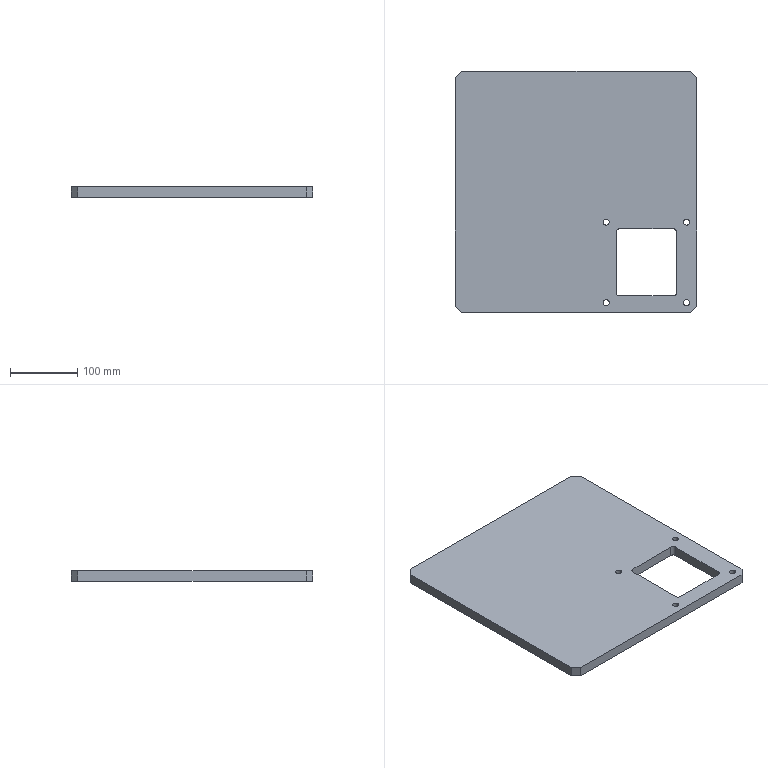Part | SolidWorks | features Chamfer 1, Extrusion 1, Fillet 1, HoleWzd 1, ICE 1 | 1 solid | 26 faces | box 360 x 360 x 15 mm | volume 1802505 mm3 | plane 14 | cylinder 12 | commonest cylinder face diameters 9 x8 10 x4
STEP:
#1=CARTESIAN_POINT('',(160.5,-45.,0.));
#2=VERTEX_POINT('',#1);
#3=CARTESIAN_POINT('',(169.5,-45.,0.));
#4=VERTEX_POINT('',#3);
#5=CARTESIAN_POINT('',(165.,-45.,0.));
#6=DIRECTION('',(0.,0.,1.));
#7=DIRECTION('',(1.,0.,0.));
#8=AXIS2_PLACEMENT_3D('',#5,#6,#7);
#9=CIRCLE('',#8,4.5);
#10=EDGE_CURVE('',#2,#4,#9,.T.);
#11=ORIENTED_EDGE('',*,*,#10,.F.);
#12=CARTESIAN_POINT('',(160.5,-45.,15.));
#13=VERTEX_POINT('',#12);
#14=CARTESIAN_POINT('',(160.5,-45.,15.));
#15=DIRECTION('',(0.,0.,1.));
#16=VECTOR('',#15,1000.);
#17=LINE('',#14,#16);
#18=EDGE_CURVE('',#2,#13,#17,.T.);
#19=ORIENTED_EDGE('',*,*,#18,.T.);
#20=CARTESIAN_POINT('',(169.5,-45.,15.));
#21=VERTEX_POINT('',#20);
#22=CARTESIAN_POINT('',(165.,-45.,15.));
#23=DIRECTION('',(0.,0.,1.));
#24=DIRECTION('',(1.,0.,0.));
#25=AXIS2_PLACEMENT_3D('',#22,#23,#24);
#26=CIRCLE('',#25,4.5);
#27=EDGE_CURVE('',#13,#21,#26,.T.);
#28=ORIENTED_EDGE('',*,*,#27,.T.);
#29=CARTESIAN_POINT('',(169.5,-45.,15.));
#30=DIRECTION('',(0.,0.,1.));
#31=VECTOR('',#30,1000.);
#32=LINE('',#29,#31);
#33=EDGE_CURVE('',#4,#21,#32,.T.);
#34=ORIENTED_EDGE('',*,*,#33,.F.);
#35=EDGE_LOOP('',(#11,#19,#28,#34));
#36=FACE_OUTER_BOUND('',#35,.T.);
#37=CARTESIAN_POINT('',(165.,-45.,15.));
#38=DIRECTION('',(0.,0.,1.));
#39=DIRECTION('',(1.,0.,0.));
#40=AXIS2_PLACEMENT_3D('',#37,#38,#39);
#41=CYLINDRICAL_SURFACE('',#40,4.5);
#42=ADVANCED_FACE('',(#36),#41,.F.);
#43=CARTESIAN_POINT('',(40.5,-45.,0.));
#44=VERTEX_POINT('',#43);
#45=CARTESIAN_POINT('',(49.5,-45.,0.));
#46=VERTEX_POINT('',#45);
#47=CARTESIAN_POINT('',(45.,-45.,0.));
#48=DIRECTION('',(0.,0.,1.));
#49=DIRECTION('',(1.,0.,0.));
#50=AXIS2_PLACEMENT_3D('',#47,#48,#49);
#51=CIRCLE('',#50,4.5);
#52=EDGE_CURVE('',#44,#46,#51,.T.);
#53=ORIENTED_EDGE('',*,*,#52,.F.);
#54=CARTESIAN_POINT('',(40.5,-45.,15.));
#55=VERTEX_POINT('',#54);
#56=CARTESIAN_POINT('',(40.5,-45.,15.));
#57=DIRECTION('',(0.,0.,1.));
#58=VECTOR('',#57,1000.);
#59=LINE('',#56,#58);
#60=EDGE_CURVE('',#44,#55,#59,.T.);
#61=ORIENTED_EDGE('',*,*,#60,.T.);
#62=CARTESIAN_POINT('',(49.5,-45.,15.));
#63=VERTEX_POINT('',#62);
#64=CARTESIAN_POINT('',(45.,-45.,15.));
#65=DIRECTION('',(0.,0.,1.));
#66=DIRECTION('',(1.,0.,0.));
#67=AXIS2_PLACEMENT_3D('',#64,#65,#66);
#68=CIRCLE('',#67,4.5);
#69=EDGE_CURVE('',#55,#63,#68,.T.);
#70=ORIENTED_EDGE('',*,*,#69,.T.);
#71=CARTESIAN_POINT('',(49.5,-45.,15.));
#72=DIRECTION('',(0.,0.,1.));
#73=VECTOR('',#72,1000.);
#74=LINE('',#71,#73);
#75=EDGE_CURVE('',#46,#63,#74,.T.);
#76=ORIENTED_EDGE('',*,*,#75,.F.);
#77=EDGE_LOOP('',(#53,#61,#70,#76));
#78=FACE_OUTER_BOUND('',#77,.T.);
#79=CARTESIAN_POINT('',(45.,-45.,15.));
#80=DIRECTION('',(0.,0.,1.));
#81=DIRECTION('',(1.,0.,0.));
#82=AXIS2_PLACEMENT_3D('',#79,#80,#81);
#83=CYLINDRICAL_SURFACE('',#82,4.5);
#84=ADVANCED_FACE('',(#78),#83,.F.);
#85=CARTESIAN_POINT('',(40.5,-165.,0.));
#86=VERTEX_POINT('',#85);
#87=CARTESIAN_POINT('',(49.5,-165.,0.));
#88=VERTEX_POINT('',#87);
#89=CARTESIAN_POINT('',(45.,-165.,0.));
#90=DIRECTION('',(0.,0.,1.));
#91=DIRECTION('',(1.,0.,0.));
#92=AXIS2_PLACEMENT_3D('',#89,#90,#91);
#93=CIRCLE('',#92,4.5);
#94=EDGE_CURVE('',#86,#88,#93,.T.);
#95=ORIENTED_EDGE('',*,*,#94,.F.);
#96=CARTESIAN_POINT('',(40.5,-165.,15.));
#97=VERTEX_POINT('',#96);
#98=CARTESIAN_POINT('',(40.5,-165.,15.));
#99=DIRECTION('',(0.,0.,1.));
#100=VECTOR('',#99,1000.);
#101=LINE('',#98,#100);
#102=EDGE_CURVE('',#86,#97,#101,.T.);
#103=ORIENTED_EDGE('',*,*,#102,.T.);
#104=CARTESIAN_POINT('',(49.5,-165.,15.));
#105=VERTEX_POINT('',#104);
#106=CARTESIAN_POINT('',(45.,-165.,15.));
#107=DIRECTION('',(0.,0.,1.));
#108=DIRECTION('',(1.,0.,0.));
#109=AXIS2_PLACEMENT_3D('',#106,#107,#108);
#110=CIRCLE('',#109,4.5);
#111=EDGE_CURVE('',#97,#105,#110,.T.);
#112=ORIENTED_EDGE('',*,*,#111,.T.);
#113=CARTESIAN_POINT('',(49.5,-165.,15.));
#114=DIRECTION('',(0.,0.,1.));
#115=VECTOR('',#114,1000.);
#116=LINE('',#113,#115);
#117=EDGE_CURVE('',#88,#105,#116,.T.);
#118=ORIENTED_EDGE('',*,*,#117,.F.);
#119=EDGE_LOOP('',(#95,#103,#112,#118));
#120=FACE_OUTER_BOUND('',#119,.T.);
#121=CARTESIAN_POINT('',(45.,-165.,15.));
#122=DIRECTION('',(0.,0.,1.));
#123=DIRECTION('',(1.,0.,0.));
#124=AXIS2_PLACEMENT_3D('',#121,#122,#123);
#125=CYLINDRICAL_SURFACE('',#124,4.5);
#126=ADVANCED_FACE('',(#120),#125,.F.);
#127=CARTESIAN_POINT('',(160.5,-165.,0.));
#128=VERTEX_POINT('',#127);
#129=CARTESIAN_POINT('',(169.5,-165.,0.));
#130=VERTEX_POINT('',#129);
#131=CARTESIAN_POINT('',(165.,-165.,0.));
#132=DIRECTION('',(0.,0.,1.));
#133=DIRECTION('',(1.,0.,0.));
#134=AXIS2_PLACEMENT_3D('',#131,#132,#133);
#135=CIRCLE('',#134,4.5);
#136=EDGE_CURVE('',#128,#130,#135,.T.);
#137=ORIENTED_EDGE('',*,*,#136,.F.);
#138=CARTESIAN_POINT('',(160.5,-165.,15.));
#139=VERTEX_POINT('',#138);
#140=CARTESIAN_POINT('',(160.5,-165.,15.));
#141=DIRECTION('',(0.,0.,1.));
#142=VECTOR('',#141,1000.);
#143=LINE('',#140,#142);
#144=EDGE_CURVE('',#128,#139,#143,.T.);
#145=ORIENTED_EDGE('',*,*,#144,.T.);
#146=CARTESIAN_POINT('',(169.5,-165.,15.));
#147=VERTEX_POINT('',#146);
#148=CARTESIAN_POINT('',(165.,-165.,15.));
#149=DIRECTION('',(0.,0.,1.));
#150=DIRECTION('',(1.,0.,0.));
#151=AXIS2_PLACEMENT_3D('',#148,#149,#150);
#152=CIRCLE('',#151,4.5);
#153=EDGE_CURVE('',#139,#147,#152,.T.);
#154=ORIENTED_EDGE('',*,*,#153,.T.);
#155=CARTESIAN_POINT('',(169.5,-165.,15.));
#156=DIRECTION('',(0.,0.,1.));
#157=VECTOR('',#156,1000.);
#158=LINE('',#155,#157);
#159=EDGE_CURVE('',#130,#147,#158,.T.);
#160=ORIENTED_EDGE('',*,*,#159,.F.);
#161=EDGE_LOOP('',(#137,#145,#154,#160));
#162=FACE_OUTER_BOUND('',#161,.T.);
#163=CARTESIAN_POINT('',(165.,-165.,15.));
#164=DIRECTION('',(0.,0.,1.));
#165=DIRECTION('',(1.,0.,0.));
#166=AXIS2_PLACEMENT_3D('',#163,#164,#165);
#167=CYLINDRICAL_SURFACE('',#166,4.5);
#168=ADVANCED_FACE('',(#162),#167,.F.);
#169=CARTESIAN_POINT('',(-180.,170.,0.));
#170=VERTEX_POINT('',#169);
#171=CARTESIAN_POINT('',(-180.,-170.,0.));
#172=VERTEX_POINT('',#171);
#173=CARTESIAN_POINT('',(-180.,180.,0.));
#174=DIRECTION('',(0.,-1.,0.));
#175=VECTOR('',#174,1000.);
#176=LINE('',#173,#175);
#177=EDGE_CURVE('',#170,#172,#176,.T.);
#178=ORIENTED_EDGE('',*,*,#177,.T.);
#179=CARTESIAN_POINT('',(-180.,-170.,15.));
#180=VERTEX_POINT('',#179);
#181=CARTESIAN_POINT('',(-180.,-170.,15.));
#182=DIRECTION('',(0.,0.,1.));
#183=VECTOR('',#182,1000.);
#184=LINE('',#181,#183);
#185=EDGE_CURVE('',#172,#180,#184,.T.);
#186=ORIENTED_EDGE('',*,*,#185,.T.);
#187=CARTESIAN_POINT('',(-180.,170.,15.));
#188=VERTEX_POINT('',#187);
#189=CARTESIAN_POINT('',(-180.,180.,15.));
#190=DIRECTION('',(0.,-1.,0.));
#191=VECTOR('',#190,1000.);
#192=LINE('',#189,#191);
#193=EDGE_CURVE('',#188,#180,#192,.T.);
#194=ORIENTED_EDGE('',*,*,#193,.F.);
#195=CARTESIAN_POINT('',(-180.,170.,0.));
#196=DIRECTION('',(0.,0.,-1.));
#197=VECTOR('',#196,1000.);
#198=LINE('',#195,#197);
#199=EDGE_CURVE('',#188,#170,#198,.T.);
#200=ORIENTED_EDGE('',*,*,#199,.T.);
#201=EDGE_LOOP('',(#178,#186,#194,#200));
#202=FACE_OUTER_BOUND('',#201,.T.);
#203=CARTESIAN_POINT('',(-180.,180.,15.));
#204=DIRECTION('',(1.,0.,0.));
#205=DIRECTION('',(0.,1.,0.));
#206=AXIS2_PLACEMENT_3D('',#203,#204,#205);
#207=PLANE('',#206);
#208=ADVANCED_FACE('',(#202),#207,.F.);
#209=CARTESIAN_POINT('',(-170.,-180.,15.));
#210=VERTEX_POINT('',#209);
#211=CARTESIAN_POINT('',(170.,-180.,15.));
#212=VERTEX_POINT('',#211);
#213=CARTESIAN_POINT('',(-180.,-180.,15.));
#214=DIRECTION('',(1.,0.,0.));
#215=VECTOR('',#214,1000.);
#216=LINE('',#213,#215);
#217=EDGE_CURVE('',#210,#212,#216,.T.);
#218=ORIENTED_EDGE('',*,*,#217,.F.);
#219=CARTESIAN_POINT('',(-170.,-180.,0.));
#220=VERTEX_POINT('',#219);
#221=CARTESIAN_POINT('',(-170.,-180.,15.));
#222=DIRECTION('',(0.,0.,-1.));
#223=VECTOR('',#222,1000.);
#224=LINE('',#221,#223);
#225=EDGE_CURVE('',#210,#220,#224,.T.);
#226=ORIENTED_EDGE('',*,*,#225,.T.);
#227=CARTESIAN_POINT('',(170.,-180.,0.));
#228=VERTEX_POINT('',#227);
#229=CARTESIAN_POINT('',(-180.,-180.,0.));
#230=DIRECTION('',(1.,0.,0.));
#231=VECTOR('',#230,1000.);
#232=LINE('',#229,#231);
#233=EDGE_CURVE('',#220,#228,#232,.T.);
#234=ORIENTED_EDGE('',*,*,#233,.T.);
#235=CARTESIAN_POINT('',(170.,-180.,15.));
#236=DIRECTION('',(0.,0.,1.));
#237=VECTOR('',#236,1000.);
#238=LINE('',#235,#237);
#239=EDGE_CURVE('',#228,#212,#238,.T.);
#240=ORIENTED_EDGE('',*,*,#239,.T.);
#241=EDGE_LOOP('',(#218,#226,#234,#240));
#242=FACE_OUTER_BOUND('',#241,.T.);
#243=CARTESIAN_POINT('',(-180.,-180.,15.));
#244=DIRECTION('',(0.,1.,0.));
#245=DIRECTION('',(0.,0.,1.));
#246=AXIS2_PLACEMENT_3D('',#243,#244,#245);
#247=PLANE('',#246);
#248=ADVANCED_FACE('',(#242),#247,.F.);
#249=CARTESIAN_POINT('',(180.,170.,15.));
#250=VERTEX_POINT('',#249);
#251=CARTESIAN_POINT('',(180.,-170.,15.));
#252=VERTEX_POINT('',#251);
#253=CARTESIAN_POINT('',(180.,180.,15.));
#254=DIRECTION('',(0.,-1.,0.));
#255=VECTOR('',#254,1000.);
#256=LINE('',#253,#255);
#257=EDGE_CURVE('',#250,#252,#256,.T.);
#258=ORIENTED_EDGE('',*,*,#257,.T.);
#259=CARTESIAN_POINT('',(180.,-170.,0.));
#260=VERTEX_POINT('',#259);
#261=CARTESIAN_POINT('',(180.,-170.,0.));
#262=DIRECTION('',(0.,0.,-1.));
#263=VECTOR('',#262,1000.);
#264=LINE('',#261,#263);
#265=EDGE_CURVE('',#252,#260,#264,.T.);
#266=ORIENTED_EDGE('',*,*,#265,.T.);
#267=CARTESIAN_POINT('',(180.,170.,0.));
#268=VERTEX_POINT('',#267);
#269=CARTESIAN_POINT('',(180.,180.,0.));
#270=DIRECTION('',(0.,-1.,0.));
#271=VECTOR('',#270,1000.);
#272=LINE('',#269,#271);
#273=EDGE_CURVE('',#268,#260,#272,.T.);
#274=ORIENTED_EDGE('',*,*,#273,.F.);
#275=CARTESIAN_POINT('',(180.,170.,15.));
#276=DIRECTION('',(0.,0.,1.));
#277=VECTOR('',#276,1000.);
#278=LINE('',#275,#277);
#279=EDGE_CURVE('',#268,#250,#278,.T.);
#280=ORIENTED_EDGE('',*,*,#279,.T.);
#281=EDGE_LOOP('',(#258,#266,#274,#280));
#282=FACE_OUTER_BOUND('',#281,.T.);
#283=CARTESIAN_POINT('',(180.,180.,15.));
#284=DIRECTION('',(1.,0.,0.));
#285=DIRECTION('',(0.,1.,0.));
#286=AXIS2_PLACEMENT_3D('',#283,#284,#285);
#287=PLANE('',#286);
#288=ADVANCED_FACE('',(#282),#287,.T.);
#289=CARTESIAN_POINT('',(-170.,180.,15.));
#290=VERTEX_POINT('',#289);
#291=CARTESIAN_POINT('',(170.,180.,15.));
#292=VERTEX_POINT('',#291);
#293=CARTESIAN_POINT('',(-180.,180.,15.));
#294=DIRECTION('',(1.,0.,0.));
#295=VECTOR('',#294,1000.);
#296=LINE('',#293,#295);
#297=EDGE_CURVE('',#290,#292,#296,.T.);
#298=ORIENTED_EDGE('',*,*,#297,.T.);
#299=CARTESIAN_POINT('',(170.,180.,0.));
#300=VERTEX_POINT('',#299);
#301=CARTESIAN_POINT('',(170.,180.,15.));
#302=DIRECTION('',(0.,0.,-1.));
#303=VECTOR('',#302,1000.);
#304=LINE('',#301,#303);
#305=EDGE_CURVE('',#292,#300,#304,.T.);
#306=ORIENTED_EDGE('',*,*,#305,.T.);
#307=CARTESIAN_POINT('',(-170.,180.,0.));
#308=VERTEX_POINT('',#307);
#309=CARTESIAN_POINT('',(-180.,180.,0.));
#310=DIRECTION('',(1.,0.,0.));
#311=VECTOR('',#310,1000.);
#312=LINE('',#309,#311);
#313=EDGE_CURVE('',#308,#300,#312,.T.);
#314=ORIENTED_EDGE('',*,*,#313,.F.);
#315=CARTESIAN_POINT('',(-170.,180.,15.));
#316=DIRECTION('',(0.,0.,1.));
#317=VECTOR('',#316,1000.);
#318=LINE('',#315,#317);
#319=EDGE_CURVE('',#308,#290,#318,.T.);
#320=ORIENTED_EDGE('',*,*,#319,.T.);
#321=EDGE_LOOP('',(#298,#306,#314,#320));
#322=FACE_OUTER_BOUND('',#321,.T.);
#323=CARTESIAN_POINT('',(-180.,180.,15.));
#324=DIRECTION('',(0.,1.,0.));
#325=DIRECTION('',(0.,0.,1.));
#326=AXIS2_PLACEMENT_3D('',#323,#324,#325);
#327=PLANE('',#326);
#328=ADVANCED_FACE('',(#322),#327,.T.);
#329=CARTESIAN_POINT('',(150.,-150.,15.));
#330=VERTEX_POINT('',#329);
#331=CARTESIAN_POINT('',(150.,-60.,15.));
#332=VERTEX_POINT('',#331);
#333=CARTESIAN_POINT('',(150.,-55.,15.));
#334=DIRECTION('',(0.,1.,0.));
#335=VECTOR('',#334,1000.);
#336=LINE('',#333,#335);
#337=EDGE_CURVE('',#330,#332,#336,.T.);
#338=ORIENTED_EDGE('',*,*,#337,.F.);
#339=CARTESIAN_POINT('',(145.,-155.,15.));
#340=VERTEX_POINT('',#339);
#341=CARTESIAN_POINT('',(145.,-150.,15.));
#342=DIRECTION('',(0.,0.,-1.));
#343=DIRECTION('',(1.,0.,0.));
#344=AXIS2_PLACEMENT_3D('',#341,#342,#343);
#345=CIRCLE('',#344,5.);
#346=EDGE_CURVE('',#330,#340,#345,.T.);
#347=ORIENTED_EDGE('',*,*,#346,.T.);
#348=CARTESIAN_POINT('',(65.,-155.,15.));
#349=VERTEX_POINT('',#348);
#350=CARTESIAN_POINT('',(60.,-155.,15.));
#351=DIRECTION('',(1.,0.,0.));
#352=VECTOR('',#351,1000.);
#353=LINE('',#350,#352);
#354=EDGE_CURVE('',#349,#340,#353,.T.);
#355=ORIENTED_EDGE('',*,*,#354,.F.);
#356=CARTESIAN_POINT('',(60.,-150.,15.));
#357=VERTEX_POINT('',#356);
#358=CARTESIAN_POINT('',(65.,-150.,15.));
#359=DIRECTION('',(0.,0.,-1.));
#360=DIRECTION('',(1.,0.,0.));
#361=AXIS2_PLACEMENT_3D('',#358,#359,#360);
#362=CIRCLE('',#361,5.);
#363=EDGE_CURVE('',#349,#357,#362,.T.);
#364=ORIENTED_EDGE('',*,*,#363,.T.);
#365=CARTESIAN_POINT('',(60.,-60.,15.));
#366=VERTEX_POINT('',#365);
#367=CARTESIAN_POINT('',(60.,-55.,15.));
#368=DIRECTION('',(0.,-1.,0.));
#369=VECTOR('',#368,1000.);
#370=LINE('',#367,#369);
#371=EDGE_CURVE('',#366,#357,#370,.T.);
#372=ORIENTED_EDGE('',*,*,#371,.F.);
#373=CARTESIAN_POINT('',(65.,-55.,15.));
#374=VERTEX_POINT('',#373);
#375=CARTESIAN_POINT('',(65.,-60.,15.));
#376=DIRECTION('',(0.,0.,-1.));
#377=DIRECTION('',(1.,0.,0.));
#378=AXIS2_PLACEMENT_3D('',#375,#376,#377);
#379=CIRCLE('',#378,5.);
#380=EDGE_CURVE('',#366,#374,#379,.T.);
#381=ORIENTED_EDGE('',*,*,#380,.T.);
#382=CARTESIAN_POINT('',(145.,-55.,15.));
#383=VERTEX_POINT('',#382);
#384=CARTESIAN_POINT('',(60.,-55.,15.));
#385=DIRECTION('',(-1.,0.,0.));
#386=VECTOR('',#385,1000.);
#387=LINE('',#384,#386);
#388=EDGE_CURVE('',#383,#374,#387,.T.);
#389=ORIENTED_EDGE('',*,*,#388,.F.);
#390=CARTESIAN_POINT('',(145.,-60.,15.));
#391=DIRECTION('',(0.,0.,-1.));
#392=DIRECTION('',(1.,0.,0.));
#393=AXIS2_PLACEMENT_3D('',#390,#391,#392);
#394=CIRCLE('',#393,5.);
#395=EDGE_CURVE('',#383,#332,#394,.T.);
#396=ORIENTED_EDGE('',*,*,#395,.T.);
#397=EDGE_LOOP('',(#338,#347,#355,#364,#372,#381,#389,#396));
#398=FACE_BOUND('',#397,.T.);
#399=CARTESIAN_POINT('',(165.,-45.,15.));
#400=DIRECTION('',(0.,0.,1.));
#401=DIRECTION('',(1.,0.,0.));
#402=AXIS2_PLACEMENT_3D('',#399,#400,#401);
#403=CIRCLE('',#402,4.5);
#404=EDGE_CURVE('',#21,#13,#403,.T.);
#405=ORIENTED_EDGE('',*,*,#404,.F.);
#406=ORIENTED_EDGE('',*,*,#27,.F.);
#407=EDGE_LOOP('',(#405,#406));
#408=FACE_BOUND('',#407,.T.);
#409=CARTESIAN_POINT('',(45.,-45.,15.));
#410=DIRECTION('',(0.,0.,1.));
#411=DIRECTION('',(1.,0.,0.));
#412=AXIS2_PLACEMENT_3D('',#409,#410,#411);
#413=CIRCLE('',#412,4.5);
#414=EDGE_CURVE('',#63,#55,#413,.T.);
#415=ORIENTED_EDGE('',*,*,#414,.F.);
#416=ORIENTED_EDGE('',*,*,#69,.F.);
#417=EDGE_LOOP('',(#415,#416));
#418=FACE_BOUND('',#417,.T.);
#419=CARTESIAN_POINT('',(45.,-165.,15.));
#420=DIRECTION('',(0.,0.,1.));
#421=DIRECTION('',(1.,0.,0.));
#422=AXIS2_PLACEMENT_3D('',#419,#420,#421);
#423=CIRCLE('',#422,4.5);
#424=EDGE_CURVE('',#105,#97,#423,.T.);
#425=ORIENTED_EDGE('',*,*,#424,.F.);
#426=ORIENTED_EDGE('',*,*,#111,.F.);
#427=EDGE_LOOP('',(#425,#426));
#428=FACE_BOUND('',#427,.T.);
#429=CARTESIAN_POINT('',(165.,-165.,15.));
#430=DIRECTION('',(0.,0.,1.));
#431=DIRECTION('',(1.,0.,0.));
#432=AXIS2_PLACEMENT_3D('',#429,#430,#431);
#433=CIRCLE('',#432,4.5);
#434=EDGE_CURVE('',#147,#139,#433,.T.);
#435=ORIENTED_EDGE('',*,*,#434,.F.);
#436=ORIENTED_EDGE('',*,*,#153,.F.);
#437=EDGE_LOOP('',(#435,#436));
#438=FACE_BOUND('',#437,.T.);
#439=ORIENTED_EDGE('',*,*,#193,.T.);
#440=CARTESIAN_POINT('',(-175.,-175.,15.));
#441=DIRECTION('',(0.7071,-0.7071,0.));
#442=VECTOR('',#441,1000.);
#443=LINE('',#440,#442);
#444=EDGE_CURVE('',#180,#210,#443,.T.);
#445=ORIENTED_EDGE('',*,*,#444,.T.);
#446=ORIENTED_EDGE('',*,*,#217,.T.);
#447=CARTESIAN_POINT('',(175.,-175.,15.));
#448=DIRECTION('',(0.7071,0.7071,0.));
#449=VECTOR('',#448,1000.);
#450=LINE('',#447,#449);
#451=EDGE_CURVE('',#212,#252,#450,.T.);
#452=ORIENTED_EDGE('',*,*,#451,.T.);
#453=ORIENTED_EDGE('',*,*,#257,.F.);
#454=CARTESIAN_POINT('',(175.,175.,15.));
#455=DIRECTION('',(-0.7071,0.7071,0.));
#456=VECTOR('',#455,1000.);
#457=LINE('',#454,#456);
#458=EDGE_CURVE('',#250,#292,#457,.T.);
#459=ORIENTED_EDGE('',*,*,#458,.T.);
#460=ORIENTED_EDGE('',*,*,#297,.F.);
#461=CARTESIAN_POINT('',(-175.,175.,15.));
#462=DIRECTION('',(-0.7071,-0.7071,0.));
#463=VECTOR('',#462,1000.);
#464=LINE('',#461,#463);
#465=EDGE_CURVE('',#290,#188,#464,.T.);
#466=ORIENTED_EDGE('',*,*,#465,.T.);
#467=EDGE_LOOP('',(#439,#445,#446,#452,#453,#459,#460,#466));
#468=FACE_OUTER_BOUND('',#467,.T.);
#469=CARTESIAN_POINT('',(0.,0.,15.));
#470=DIRECTION('',(0.,0.,1.));
#471=DIRECTION('',(1.,0.,0.));
#472=AXIS2_PLACEMENT_3D('',#469,#470,#471);
#473=PLANE('',#472);
#474=ADVANCED_FACE('',(#398,#408,#418,#428,#438,#468),#473,.T.);
#475=CARTESIAN_POINT('',(60.,-60.,0.));
#476=VERTEX_POINT('',#475);
#477=CARTESIAN_POINT('',(60.,-150.,0.));
#478=VERTEX_POINT('',#477);
#479=CARTESIAN_POINT('',(60.,-55.,0.));
#480=DIRECTION('',(0.,-1.,0.));
#481=VECTOR('',#480,1000.);
#482=LINE('',#479,#481);
#483=EDGE_CURVE('',#476,#478,#482,.T.);
#484=ORIENTED_EDGE('',*,*,#483,.T.);
#485=CARTESIAN_POINT('',(65.,-155.,0.));
#486=VERTEX_POINT('',#485);
#487=CARTESIAN_POINT('',(65.,-150.,0.));
#488=DIRECTION('',(0.,0.,1.));
#489=DIRECTION('',(1.,0.,0.));
#490=AXIS2_PLACEMENT_3D('',#487,#488,#489);
#491=CIRCLE('',#490,5.);
#492=EDGE_CURVE('',#478,#486,#491,.T.);
#493=ORIENTED_EDGE('',*,*,#492,.T.);
#494=CARTESIAN_POINT('',(145.,-155.,0.));
#495=VERTEX_POINT('',#494);
#496=CARTESIAN_POINT('',(60.,-155.,0.));
#497=DIRECTION('',(1.,0.,0.));
#498=VECTOR('',#497,1000.);
#499=LINE('',#496,#498);
#500=EDGE_CURVE('',#486,#495,#499,.T.);
#501=ORIENTED_EDGE('',*,*,#500,.T.);
#502=CARTESIAN_POINT('',(150.,-150.,0.));
#503=VERTEX_POINT('',#502);
#504=CARTESIAN_POINT('',(145.,-150.,0.));
#505=DIRECTION('',(0.,0.,1.));
#506=DIRECTION('',(1.,0.,0.));
#507=AXIS2_PLACEMENT_3D('',#504,#505,#506);
#508=CIRCLE('',#507,5.);
#509=EDGE_CURVE('',#495,#503,#508,.T.);
#510=ORIENTED_EDGE('',*,*,#509,.T.);
#511=CARTESIAN_POINT('',(150.,-60.,0.));
#512=VERTEX_POINT('',#511);
#513=CARTESIAN_POINT('',(150.,-55.,0.));
#514=DIRECTION('',(0.,1.,0.));
#515=VECTOR('',#514,1000.);
#516=LINE('',#513,#515);
#517=EDGE_CURVE('',#503,#512,#516,.T.);
#518=ORIENTED_EDGE('',*,*,#517,.T.);
#519=CARTESIAN_POINT('',(145.,-55.,0.));
#520=VERTEX_POINT('',#519);
#521=CARTESIAN_POINT('',(145.,-60.,0.));
#522=DIRECTION('',(0.,0.,1.));
#523=DIRECTION('',(1.,0.,0.));
#524=AXIS2_PLACEMENT_3D('',#521,#522,#523);
#525=CIRCLE('',#524,5.);
#526=EDGE_CURVE('',#512,#520,#525,.T.);
#527=ORIENTED_EDGE('',*,*,#526,.T.);
#528=CARTESIAN_POINT('',(65.,-55.,0.));
#529=VERTEX_POINT('',#528);
#530=CARTESIAN_POINT('',(60.,-55.,0.));
#531=DIRECTION('',(-1.,0.,0.));
#532=VECTOR('',#531,1000.);
#533=LINE('',#530,#532);
#534=EDGE_CURVE('',#520,#529,#533,.T.);
#535=ORIENTED_EDGE('',*,*,#534,.T.);
#536=CARTESIAN_POINT('',(65.,-60.,0.));
#537=DIRECTION('',(0.,0.,1.));
#538=DIRECTION('',(1.,0.,0.));
#539=AXIS2_PLACEMENT_3D('',#536,#537,#538);
#540=CIRCLE('',#539,5.);
#541=EDGE_CURVE('',#529,#476,#540,.T.);
#542=ORIENTED_EDGE('',*,*,#541,.T.);
#543=EDGE_LOOP('',(#484,#493,#501,#510,#518,#527,#535,#542));
#544=FACE_BOUND('',#543,.T.);
#545=CARTESIAN_POINT('',(165.,-45.,0.));
#546=DIRECTION('',(0.,0.,1.));
#547=DIRECTION('',(1.,0.,0.));
#548=AXIS2_PLACEMENT_3D('',#545,#546,#547);
#549=CIRCLE('',#548,4.5);
#550=EDGE_CURVE('',#4,#2,#549,.T.);
#551=ORIENTED_EDGE('',*,*,#550,.T.);
#552=ORIENTED_EDGE('',*,*,#10,.T.);
#553=EDGE_LOOP('',(#551,#552));
#554=FACE_BOUND('',#553,.T.);
#555=CARTESIAN_POINT('',(45.,-45.,0.));
#556=DIRECTION('',(0.,0.,1.));
#557=DIRECTION('',(1.,0.,0.));
#558=AXIS2_PLACEMENT_3D('',#555,#556,#557);
#559=CIRCLE('',#558,4.5);
#560=EDGE_CURVE('',#46,#44,#559,.T.);
#561=ORIENTED_EDGE('',*,*,#560,.T.);
#562=ORIENTED_EDGE('',*,*,#52,.T.);
#563=EDGE_LOOP('',(#561,#562));
#564=FACE_BOUND('',#563,.T.);
#565=CARTESIAN_POINT('',(45.,-165.,0.));
#566=DIRECTION('',(0.,0.,1.));
#567=DIRECTION('',(1.,0.,0.));
#568=AXIS2_PLACEMENT_3D('',#565,#566,#567);
#569=CIRCLE('',#568,4.5);
#570=EDGE_CURVE('',#88,#86,#569,.T.);
#571=ORIENTED_EDGE('',*,*,#570,.T.);
#572=ORIENTED_EDGE('',*,*,#94,.T.);
#573=EDGE_LOOP('',(#571,#572));
#574=FACE_BOUND('',#573,.T.);
#575=CARTESIAN_POINT('',(165.,-165.,0.));
#576=DIRECTION('',(0.,0.,1.));
#577=DIRECTION('',(1.,0.,0.));
#578=AXIS2_PLACEMENT_3D('',#575,#576,#577);
#579=CIRCLE('',#578,4.5);
#580=EDGE_CURVE('',#130,#128,#579,.T.);
#581=ORIENTED_EDGE('',*,*,#580,.T.);
#582=ORIENTED_EDGE('',*,*,#136,.T.);
#583=EDGE_LOOP('',(#581,#582));
#584=FACE_BOUND('',#583,.T.);
#585=ORIENTED_EDGE('',*,*,#233,.F.);
#586=CARTESIAN_POINT('',(-170.,-180.,0.));
#587=DIRECTION('',(-0.7071,0.7071,0.));
#588=VECTOR('',#587,1000.);
#589=LINE('',#586,#588);
#590=EDGE_CURVE('',#220,#172,#589,.T.);
#591=ORIENTED_EDGE('',*,*,#590,.T.);
#592=ORIENTED_EDGE('',*,*,#177,.F.);
#593=CARTESIAN_POINT('',(-180.,170.,0.));
#594=DIRECTION('',(0.7071,0.7071,0.));
#595=VECTOR('',#594,1000.);
#596=LINE('',#593,#595);
#597=EDGE_CURVE('',#170,#308,#596,.T.);
#598=ORIENTED_EDGE('',*,*,#597,.T.);
#599=ORIENTED_EDGE('',*,*,#313,.T.);
#600=CARTESIAN_POINT('',(170.,180.,0.));
#601=DIRECTION('',(0.7071,-0.7071,0.));
#602=VECTOR('',#601,1000.);
#603=LINE('',#600,#602);
#604=EDGE_CURVE('',#300,#268,#603,.T.);
#605=ORIENTED_EDGE('',*,*,#604,.T.);
#606=ORIENTED_EDGE('',*,*,#273,.T.);
#607=CARTESIAN_POINT('',(180.,-170.,0.));
#608=DIRECTION('',(-0.7071,-0.7071,0.));
#609=VECTOR('',#608,1000.);
#610=LINE('',#607,#609);
#611=EDGE_CURVE('',#260,#228,#610,.T.);
#612=ORIENTED_EDGE('',*,*,#611,.T.);
#613=EDGE_LOOP('',(#585,#591,#592,#598,#599,#605,#606,#612));
#614=FACE_OUTER_BOUND('',#613,.T.);
#615=CARTESIAN_POINT('',(0.,0.,0.));
#616=DIRECTION('',(0.,0.,1.));
#617=DIRECTION('',(1.,0.,0.));
#618=AXIS2_PLACEMENT_3D('',#615,#616,#617);
#619=PLANE('',#618);
#620=ADVANCED_FACE('',(#544,#554,#564,#574,#584,#614),#619,.F.);
#621=ORIENTED_EDGE('',*,*,#444,.F.);
#622=ORIENTED_EDGE('',*,*,#185,.F.);
#623=ORIENTED_EDGE('',*,*,#590,.F.);
#624=ORIENTED_EDGE('',*,*,#225,.F.);
#625=EDGE_LOOP('',(#621,#622,#623,#624));
#626=FACE_OUTER_BOUND('',#625,.T.);
#627=CARTESIAN_POINT('',(-170.,-180.,15.));
#628=DIRECTION('',(0.7071,0.7071,0.));
#629=DIRECTION('',(0.,0.,-1.));
#630=AXIS2_PLACEMENT_3D('',#627,#628,#629);
#631=PLANE('',#630);
#632=ADVANCED_FACE('',(#626),#631,.F.);
#633=ORIENTED_EDGE('',*,*,#451,.F.);
#634=ORIENTED_EDGE('',*,*,#239,.F.);
#635=ORIENTED_EDGE('',*,*,#611,.F.);
#636=ORIENTED_EDGE('',*,*,#265,.F.);
#637=EDGE_LOOP('',(#633,#634,#635,#636));
#638=FACE_OUTER_BOUND('',#637,.T.);
#639=CARTESIAN_POINT('',(180.,-170.,15.));
#640=DIRECTION('',(0.7071,-0.7071,0.));
#641=DIRECTION('',(0.,0.,1.));
#642=AXIS2_PLACEMENT_3D('',#639,#640,#641);
#643=PLANE('',#642);
#644=ADVANCED_FACE('',(#638),#643,.T.);
#645=ORIENTED_EDGE('',*,*,#458,.F.);
#646=ORIENTED_EDGE('',*,*,#279,.F.);
#647=ORIENTED_EDGE('',*,*,#604,.F.);
#648=ORIENTED_EDGE('',*,*,#305,.F.);
#649=EDGE_LOOP('',(#645,#646,#647,#648));
#650=FACE_OUTER_BOUND('',#649,.T.);
#651=CARTESIAN_POINT('',(170.,180.,15.));
#652=DIRECTION('',(-0.7071,-0.7071,0.));
#653=DIRECTION('',(0.,0.,-1.));
#654=AXIS2_PLACEMENT_3D('',#651,#652,#653);
#655=PLANE('',#654);
#656=ADVANCED_FACE('',(#650),#655,.F.);
#657=ORIENTED_EDGE('',*,*,#465,.F.);
#658=ORIENTED_EDGE('',*,*,#319,.F.);
#659=ORIENTED_EDGE('',*,*,#597,.F.);
#660=ORIENTED_EDGE('',*,*,#199,.F.);
#661=EDGE_LOOP('',(#657,#658,#659,#660));
#662=FACE_OUTER_BOUND('',#661,.T.);
#663=CARTESIAN_POINT('',(-180.,170.,15.));
#664=DIRECTION('',(-0.7071,0.7071,0.));
#665=DIRECTION('',(0.,0.,1.));
#666=AXIS2_PLACEMENT_3D('',#663,#664,#665);
#667=PLANE('',#666);
#668=ADVANCED_FACE('',(#662),#667,.T.);
#669=ORIENTED_EDGE('',*,*,#144,.F.);
#670=ORIENTED_EDGE('',*,*,#580,.F.);
#671=ORIENTED_EDGE('',*,*,#159,.T.);
#672=ORIENTED_EDGE('',*,*,#434,.T.);
#673=EDGE_LOOP('',(#669,#670,#671,#672));
#674=FACE_OUTER_BOUND('',#673,.T.);
#675=CARTESIAN_POINT('',(165.,-165.,15.));
#676=DIRECTION('',(0.,0.,1.));
#677=DIRECTION('',(1.,0.,0.));
#678=AXIS2_PLACEMENT_3D('',#675,#676,#677);
#679=CYLINDRICAL_SURFACE('',#678,4.5);
#680=ADVANCED_FACE('',(#674),#679,.F.);
#681=ORIENTED_EDGE('',*,*,#102,.F.);
#682=ORIENTED_EDGE('',*,*,#570,.F.);
#683=ORIENTED_EDGE('',*,*,#117,.T.);
#684=ORIENTED_EDGE('',*,*,#424,.T.);
#685=EDGE_LOOP('',(#681,#682,#683,#684));
#686=FACE_OUTER_BOUND('',#685,.T.);
#687=CARTESIAN_POINT('',(45.,-165.,15.));
#688=DIRECTION('',(0.,0.,1.));
#689=DIRECTION('',(1.,0.,0.));
#690=AXIS2_PLACEMENT_3D('',#687,#688,#689);
#691=CYLINDRICAL_SURFACE('',#690,4.5);
#692=ADVANCED_FACE('',(#686),#691,.F.);
#693=ORIENTED_EDGE('',*,*,#60,.F.);
#694=ORIENTED_EDGE('',*,*,#560,.F.);
#695=ORIENTED_EDGE('',*,*,#75,.T.);
#696=ORIENTED_EDGE('',*,*,#414,.T.);
#697=EDGE_LOOP('',(#693,#694,#695,#696));
#698=FACE_OUTER_BOUND('',#697,.T.);
#699=CARTESIAN_POINT('',(45.,-45.,15.));
#700=DIRECTION('',(0.,0.,1.));
#701=DIRECTION('',(1.,0.,0.));
#702=AXIS2_PLACEMENT_3D('',#699,#700,#701);
#703=CYLINDRICAL_SURFACE('',#702,4.5);
#704=ADVANCED_FACE('',(#698),#703,.F.);
#705=ORIENTED_EDGE('',*,*,#18,.F.);
#706=ORIENTED_EDGE('',*,*,#550,.F.);
#707=ORIENTED_EDGE('',*,*,#33,.T.);
#708=ORIENTED_EDGE('',*,*,#404,.T.);
#709=EDGE_LOOP('',(#705,#706,#707,#708));
#710=FACE_OUTER_BOUND('',#709,.T.);
#711=CARTESIAN_POINT('',(165.,-45.,15.));
#712=DIRECTION('',(0.,0.,1.));
#713=DIRECTION('',(1.,0.,0.));
#714=AXIS2_PLACEMENT_3D('',#711,#712,#713);
#715=CYLINDRICAL_SURFACE('',#714,4.5);
#716=ADVANCED_FACE('',(#710),#715,.F.);
#717=ORIENTED_EDGE('',*,*,#517,.F.);
#718=CARTESIAN_POINT('',(150.,-150.,15.));
#719=DIRECTION('',(0.,0.,1.));
#720=VECTOR('',#719,1000.);
#721=LINE('',#718,#720);
#722=EDGE_CURVE('',#503,#330,#721,.T.);
#723=ORIENTED_EDGE('',*,*,#722,.T.);
#724=ORIENTED_EDGE('',*,*,#337,.T.);
#725=CARTESIAN_POINT('',(150.,-60.,0.));
#726=DIRECTION('',(0.,0.,-1.));
#727=VECTOR('',#726,1000.);
#728=LINE('',#725,#727);
#729=EDGE_CURVE('',#332,#512,#728,.T.);
#730=ORIENTED_EDGE('',*,*,#729,.T.);
#731=EDGE_LOOP('',(#717,#723,#724,#730));
#732=FACE_OUTER_BOUND('',#731,.T.);
#733=CARTESIAN_POINT('',(150.,-55.,0.));
#734=DIRECTION('',(1.,0.,0.));
#735=DIRECTION('',(0.,0.,-1.));
#736=AXIS2_PLACEMENT_3D('',#733,#734,#735);
#737=PLANE('',#736);
#738=ADVANCED_FACE('',(#732),#737,.F.);
#739=ORIENTED_EDGE('',*,*,#354,.T.);
#740=CARTESIAN_POINT('',(145.,-155.,0.));
#741=DIRECTION('',(0.,0.,-1.));
#742=VECTOR('',#741,1000.);
#743=LINE('',#740,#742);
#744=EDGE_CURVE('',#340,#495,#743,.T.);
#745=ORIENTED_EDGE('',*,*,#744,.T.);
#746=ORIENTED_EDGE('',*,*,#500,.F.);
#747=CARTESIAN_POINT('',(65.,-155.,15.));
#748=DIRECTION('',(0.,0.,1.));
#749=VECTOR('',#748,1000.);
#750=LINE('',#747,#749);
#751=EDGE_CURVE('',#486,#349,#750,.T.);
#752=ORIENTED_EDGE('',*,*,#751,.T.);
#753=EDGE_LOOP('',(#739,#745,#746,#752));
#754=FACE_OUTER_BOUND('',#753,.T.);
#755=CARTESIAN_POINT('',(60.,-155.,0.));
#756=DIRECTION('',(0.,-1.,0.));
#757=DIRECTION('',(0.,0.,-1.));
#758=AXIS2_PLACEMENT_3D('',#755,#756,#757);
#759=PLANE('',#758);
#760=ADVANCED_FACE('',(#754),#759,.F.);
#761=ORIENTED_EDGE('',*,*,#371,.T.);
#762=CARTESIAN_POINT('',(60.,-150.,0.));
#763=DIRECTION('',(0.,0.,-1.));
#764=VECTOR('',#763,1000.);
#765=LINE('',#762,#764);
#766=EDGE_CURVE('',#357,#478,#765,.T.);
#767=ORIENTED_EDGE('',*,*,#766,.T.);
#768=ORIENTED_EDGE('',*,*,#483,.F.);
#769=CARTESIAN_POINT('',(60.,-60.,15.));
#770=DIRECTION('',(0.,0.,1.));
#771=VECTOR('',#770,1000.);
#772=LINE('',#769,#771);
#773=EDGE_CURVE('',#476,#366,#772,.T.);
#774=ORIENTED_EDGE('',*,*,#773,.T.);
#775=EDGE_LOOP('',(#761,#767,#768,#774));
#776=FACE_OUTER_BOUND('',#775,.T.);
#777=CARTESIAN_POINT('',(60.,-55.,0.));
#778=DIRECTION('',(-1.,0.,0.));
#779=DIRECTION('',(0.,-1.,0.));
#780=AXIS2_PLACEMENT_3D('',#777,#778,#779);
#781=PLANE('',#780);
#782=ADVANCED_FACE('',(#776),#781,.F.);
#783=ORIENTED_EDGE('',*,*,#534,.F.);
#784=CARTESIAN_POINT('',(145.,-55.,15.));
#785=DIRECTION('',(0.,0.,1.));
#786=VECTOR('',#785,1000.);
#787=LINE('',#784,#786);
#788=EDGE_CURVE('',#520,#383,#787,.T.);
#789=ORIENTED_EDGE('',*,*,#788,.T.);
#790=ORIENTED_EDGE('',*,*,#388,.T.);
#791=CARTESIAN_POINT('',(65.,-55.,0.));
#792=DIRECTION('',(0.,0.,-1.));
#793=VECTOR('',#792,1000.);
#794=LINE('',#791,#793);
#795=EDGE_CURVE('',#374,#529,#794,.T.);
#796=ORIENTED_EDGE('',*,*,#795,.T.);
#797=EDGE_LOOP('',(#783,#789,#790,#796));
#798=FACE_OUTER_BOUND('',#797,.T.);
#799=CARTESIAN_POINT('',(60.,-55.,0.));
#800=DIRECTION('',(0.,1.,0.));
#801=DIRECTION('',(0.,0.,1.));
#802=AXIS2_PLACEMENT_3D('',#799,#800,#801);
#803=PLANE('',#802);
#804=ADVANCED_FACE('',(#798),#803,.F.);
#805=ORIENTED_EDGE('',*,*,#509,.F.);
#806=ORIENTED_EDGE('',*,*,#744,.F.);
#807=ORIENTED_EDGE('',*,*,#346,.F.);
#808=ORIENTED_EDGE('',*,*,#722,.F.);
#809=EDGE_LOOP('',(#805,#806,#807,#808));
#810=FACE_OUTER_BOUND('',#809,.T.);
#811=CARTESIAN_POINT('',(145.,-150.,0.));
#812=DIRECTION('',(0.,0.,-1.));
#813=DIRECTION('',(-1.,0.,0.));
#814=AXIS2_PLACEMENT_3D('',#811,#812,#813);
#815=CYLINDRICAL_SURFACE('',#814,5.);
#816=ADVANCED_FACE('',(#810),#815,.F.);
#817=ORIENTED_EDGE('',*,*,#492,.F.);
#818=ORIENTED_EDGE('',*,*,#766,.F.);
#819=ORIENTED_EDGE('',*,*,#363,.F.);
#820=ORIENTED_EDGE('',*,*,#751,.F.);
#821=EDGE_LOOP('',(#817,#818,#819,#820));
#822=FACE_OUTER_BOUND('',#821,.T.);
#823=CARTESIAN_POINT('',(65.,-150.,0.));
#824=DIRECTION('',(0.,0.,-1.));
#825=DIRECTION('',(-1.,0.,0.));
#826=AXIS2_PLACEMENT_3D('',#823,#824,#825);
#827=CYLINDRICAL_SURFACE('',#826,5.);
#828=ADVANCED_FACE('',(#822),#827,.F.);
#829=ORIENTED_EDGE('',*,*,#526,.F.);
#830=ORIENTED_EDGE('',*,*,#729,.F.);
#831=ORIENTED_EDGE('',*,*,#395,.F.);
#832=ORIENTED_EDGE('',*,*,#788,.F.);
#833=EDGE_LOOP('',(#829,#830,#831,#832));
#834=FACE_OUTER_BOUND('',#833,.T.);
#835=CARTESIAN_POINT('',(145.,-60.,0.));
#836=DIRECTION('',(0.,0.,-1.));
#837=DIRECTION('',(-1.,0.,0.));
#838=AXIS2_PLACEMENT_3D('',#835,#836,#837);
#839=CYLINDRICAL_SURFACE('',#838,5.);
#840=ADVANCED_FACE('',(#834),#839,.F.);
#841=ORIENTED_EDGE('',*,*,#541,.F.);
#842=ORIENTED_EDGE('',*,*,#795,.F.);
#843=ORIENTED_EDGE('',*,*,#380,.F.);
#844=ORIENTED_EDGE('',*,*,#773,.F.);
#845=EDGE_LOOP('',(#841,#842,#843,#844));
#846=FACE_OUTER_BOUND('',#845,.T.);
#847=CARTESIAN_POINT('',(65.,-60.,0.));
#848=DIRECTION('',(0.,0.,-1.));
#849=DIRECTION('',(-1.,0.,0.));
#850=AXIS2_PLACEMENT_3D('',#847,#848,#849);
#851=CYLINDRICAL_SURFACE('',#850,5.);
#852=ADVANCED_FACE('',(#846),#851,.F.);
#853=CLOSED_SHELL('',(#42,#84,#126,#168,#208,#248,#288,#328,#474,#620,#632,#644,#656,#668,#680,#692,#704,#716,#738,#760,#782,#804,#816,#828,#840,#852));
#854=MANIFOLD_SOLID_BREP('',#853);
#855=CARTESIAN_POINT('',(0.,0.,0.));
#856=DIRECTION('',(0.,0.,1.));
#857=DIRECTION('',(1.,0.,0.));
#858=AXIS2_PLACEMENT_3D('',#855,#856,#857);
#859=(LENGTH_UNIT()NAMED_UNIT(*)SI_UNIT(.MILLI.,.METRE.));
#860=UNCERTAINTY_MEASURE_WITH_UNIT(LENGTH_MEASURE(0.00001),#859,'','');
#861=(NAMED_UNIT(*)PLANE_ANGLE_UNIT()SI_UNIT($,.RADIAN.));
#862=(NAMED_UNIT(*)SI_UNIT($,.STERADIAN.)SOLID_ANGLE_UNIT());
#863=(GEOMETRIC_REPRESENTATION_CONTEXT(3)GLOBAL_UNCERTAINTY_ASSIGNED_CONTEXT((#860))GLOBAL_UNIT_ASSIGNED_CONTEXT((#859,#861,#862))REPRESENTATION_CONTEXT('',''));
#864=ADVANCED_BREP_SHAPE_REPRESENTATION('',(#854,#858),#863);